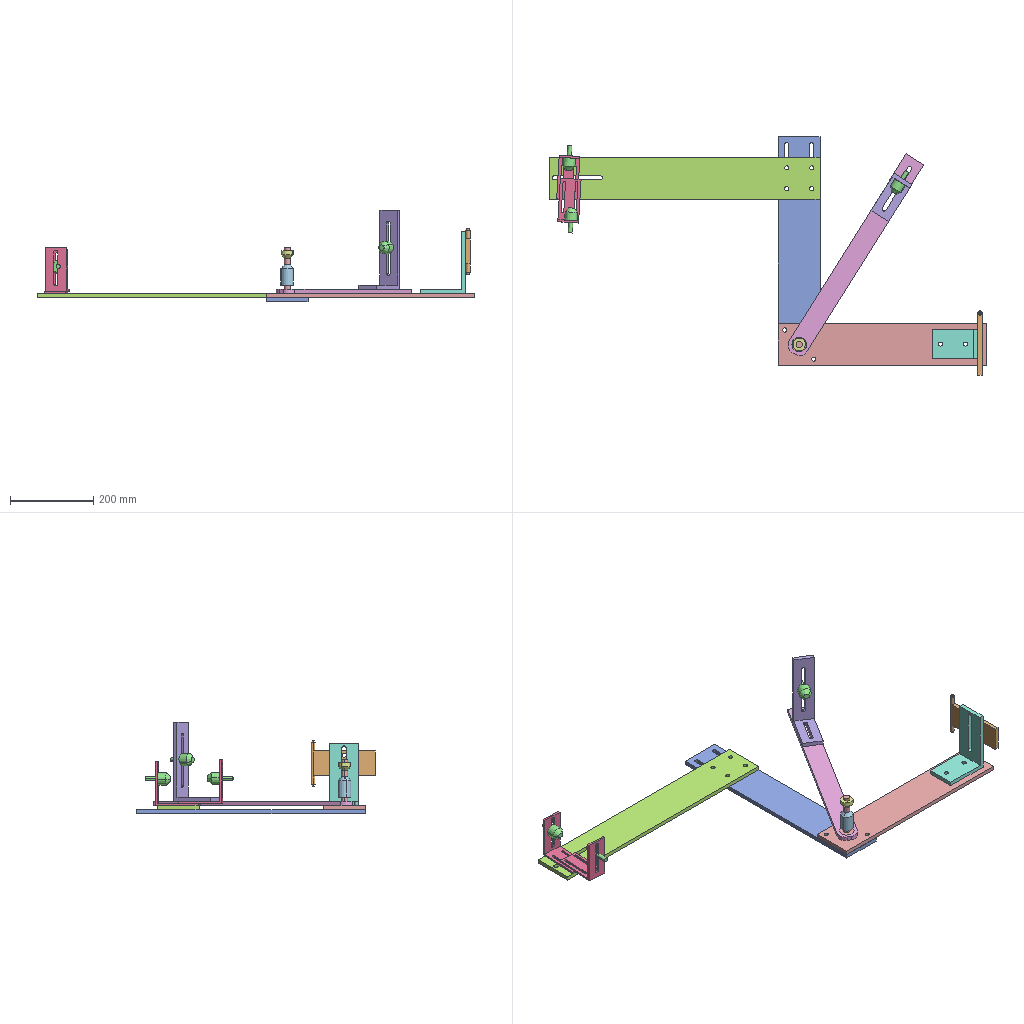Assembly | SolidWorks | 12 different items | 15 placed | box 1050 x 574 x 220 mm
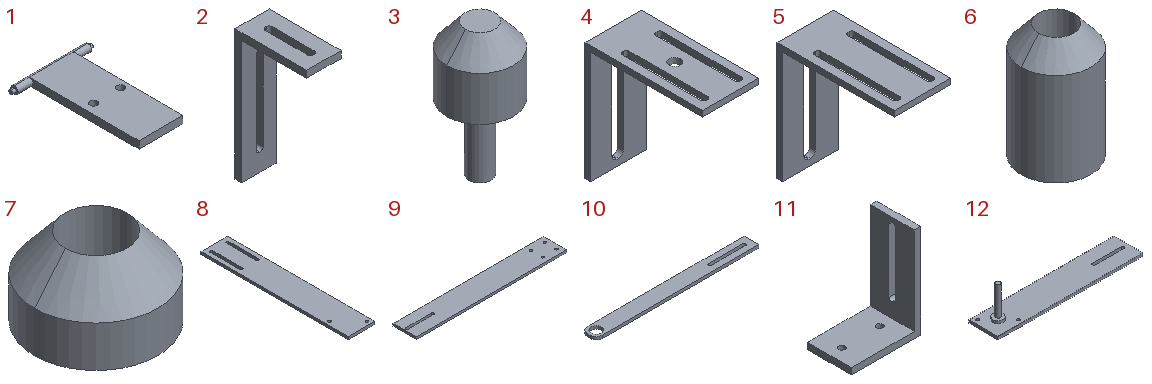Parts list (item | quantity | size | volume | features):
1 | x1 | 110 x 155 x 10 mm | 94123 mm3 | features ICE 3, Extrusion 1
2 | x1 | 50 x 105 x 190 mm | 122848 mm3 | features ICE 3, Extrusion 1
3 | x3 | 30 x 30 x 60 mm | 20345 mm3 | features Chamfer 1, Extrusion 1, ICE 1
4 | x1 | 50 x 105 x 105 mm | 42248 mm3 | features ICE 4, Extrusion 1
5 | x2 | 50 x 105 x 105 mm | 42641 mm3 | features ICE 3, Extrusion 1
6 | x1 | 30 x 30 x 48.938 mm | 23312 mm3 | features Chamfer 1, Extrusion 1
7 | x1 | 30 x 30 x 18.938 mm | 7407 mm3 | features Chamfer 1, Extrusion 1
8 | x1 | 100 x 550 x 10 mm | 524777 mm3 | features ICE 2, Extrusion 1
9 | x1 | 650 x 100 x 10 mm | 635032 mm3 | features ICE 2, Extrusion 1
10 | x1 | 550 x 50 x 10 mm | 251336 mm3 | features ICE 2, Extrusion 1, Fillet 1
11 | x1 | 110 x 70 x 150 mm | 162603 mm3 | features ICE 3, Extrusion 1
12 | x1 | 500 x 100 x 120 mm | 514971 mm3 | features ICE 5, Extrusion 1
Mates (type | each side: item.copy, entity, surface, feature):
Coincident | 12.1 edge | 8.1 edge | 2 times
Coincident | 8.1 edge | 9.1 edge
Coincident | 8.1 face plane Boss-Extrude1 | 9.1 face plane Boss-Extrude1
Concentric | 12.1 face cylinder Boss-Extrude2 | 10.1 face cylinder Cut-Extrude1
Coincident | 12.1 edge | 10.1 edge
Coincident | 12.1 face plane Boss-Extrude1 | 11.1 face plane Boss-Extrude1
Coincident | 11.1 face plane Boss-Extrude2 | 1.1 face plane Boss-Extrude1
Coincident | 10.1 face plane Boss-Extrude1 | 2.1 face plane Boss-Extrude1
Coincident | 10.1 edge | 2.1 edge | 2 times
Coincident | 2.1 face plane Boss-Extrude2 | 3.1 face plane Boss-Extrude2
Coincident | 9.1 face plane Boss-Extrude1 | 5.1 face plane Boss-Extrude1
Coincident | 5.1 face plane Boss-Extrude1 | 5.2 face plane Boss-Extrude1
Coincident | 5.1 face plane Boss-Extrude2 | 3.2 face plane Boss-Extrude2
Coincident | 5.2 face plane Boss-Extrude2 | 3.3 face plane Boss-Extrude2
Concentric | 12.1 face cylinder Cut-Extrude3 | 6.1 face cylinder Boss-Extrude1
Concentric | 12.1 face cylinder Cut-Extrude3 | 7.1 face cylinder Boss-Extrude1